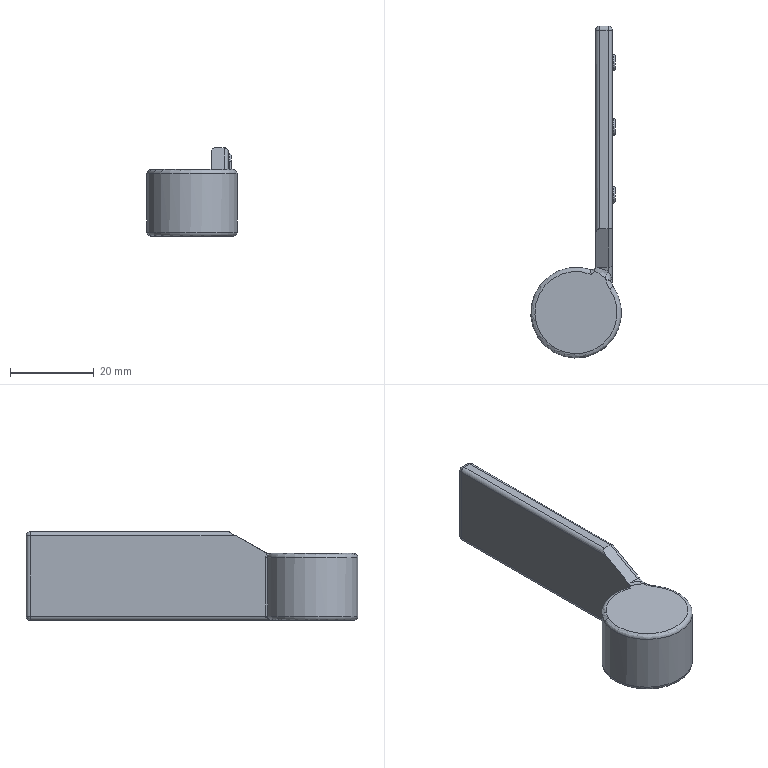Part | STEP file | DEWALT-DWE7492-B2_002 | 1 solid | 61 faces | box 21.679 x 79.466 x 21.2 mm | volume 10933 mm3 | cylinder 25 | plane 17 | torus 9 | spline 6 | sphere 4 | commonest cylinder face diameters 2 x11 4 x7 1 x6 21.679 x1